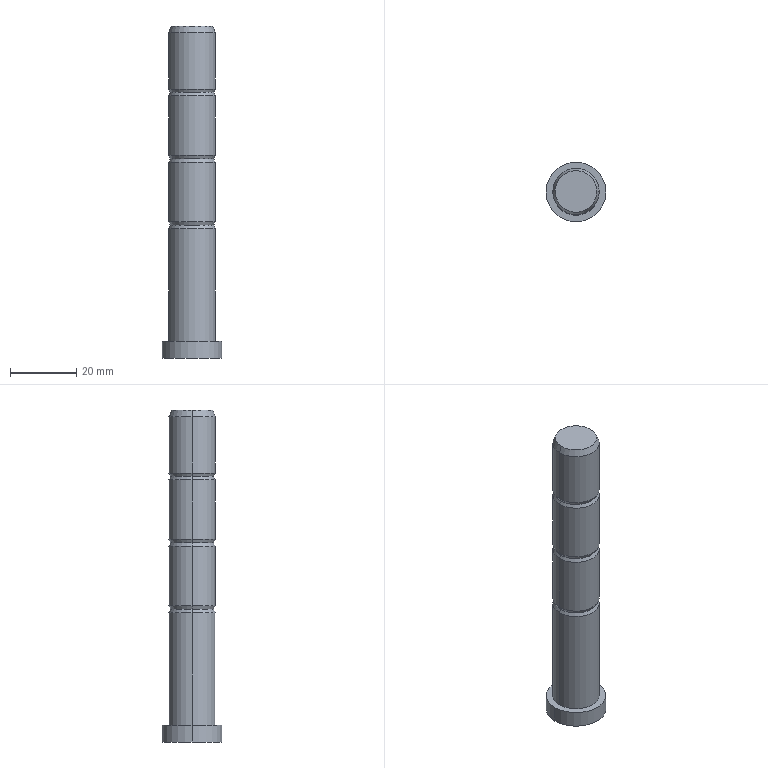Part | STEP file | EES - 2C 12x100_2 | 1 solid | 27 faces | box 18 x 18 x 100 mm | volume 15801 mm3 | cone 14 | cylinder 10 | plane 3 | commonest cylinder face diameters 14 x8 18 x2